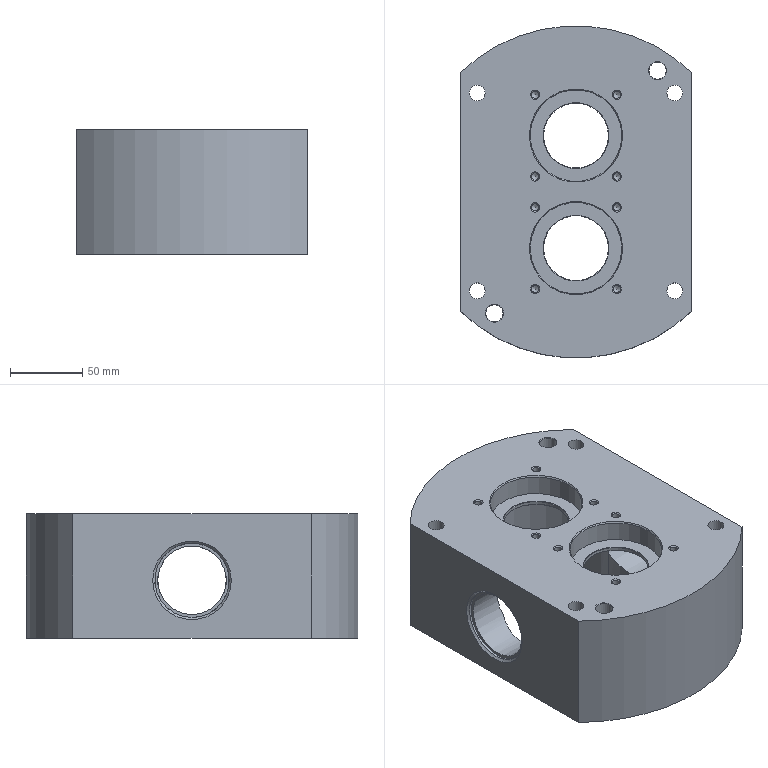NC program | NX | posted with a generic post | part box 160 x 230 x 86 mm
Lines 86 to 894 of 2142:
(HOLE_MILLING_COPY_COPY , TOOL : D10)
N146 T10 M6
N148 G54
N150 G17 G0 G90 X-39. Y0. B0. C0. S3000 M3
N152 G43 Z30. H10
N154 Z0.5
N156 G94 G3 X-40.25 Y-1.25 R1.25 F2200.
N158 X-39. Y-2.5 R1.25
N160 X-39. Y-2.5 Z0.28 I0. J2.5
N162 X-39. Y-2.5 Z0.06 I0. J2.5
N164 X-39. Y-2.5 Z-0.16 I0. J2.5
N166 X-39. Y-2.5 Z-0.38 I0. J2.5
N168 X-39. Y-2.5 Z-0.6 I0. J2.5
N170 X-39. Y-2.5 Z-0.82 I0. J2.5
N172 X-39. Y-2.5 Z-1.04 I0. J2.5
N174 X-39. Y-2.5 Z-1.26 I0. J2.5
N176 X-39. Y-2.5 Z-1.48 I0. J2.5
N178 X-39. Y-2.5 Z-1.7 I0. J2.5
N180 X-39. Y-2.5 Z-1.92 I0. J2.5
N182 X-39. Y-2.5 Z-2.14 I0. J2.5
N184 X-39. Y-2.5 Z-2.36 I0. J2.5
N186 X-39. Y-2.5 Z-2.58 I0. J2.5
N188 X-39. Y-2.5 Z-2.8 I0. J2.5
N190 X-39. Y-2.5 Z-3.02 I0. J2.5
N192 X-39. Y-2.5 Z-3.24 I0. J2.5
N194 X-39. Y-2.5 Z-3.46 I0. J2.5
N196 X-39. Y-2.5 Z-3.68 I0. J2.5
N198 X-39. Y-2.5 Z-3.9 I0. J2.5
N200 X-39. Y-2.5 Z-4.12 I0. J2.5
N202 X-39. Y-2.5 Z-4.34 I0. J2.5
N204 X-39. Y-2.5 Z-4.56 I0. J2.5
N206 X-39. Y-2.5 Z-4.78 I0. J2.5
N208 X-39. Y-2.5 Z-5. I0. J2.5
N210 X-39. Y-2.5 Z-5.22 I0. J2.5
N212 X-39. Y-2.5 Z-5.44 I0. J2.5
N214 X-39. Y-2.5 Z-5.66 I0. J2.5
N216 X-39. Y-2.5 Z-5.88 I0. J2.5
N218 X-39. Y-2.5 Z-6.1 I0. J2.5
N220 X-39. Y-2.5 Z-6.32 I0. J2.5
N222 X-39. Y-2.5 Z-6.54 I0. J2.5
N224 X-39. Y-2.5 Z-6.76 I0. J2.5
N226 X-39. Y-2.5 Z-6.98 I0. J2.5
N228 X-39. Y-2.5 Z-7.2 I0. J2.5
N230 X-39. Y-2.5 Z-7.42 I0. J2.5
N232 X-39. Y-2.5 Z-7.64 I0. J2.5
N234 X-39. Y-2.5 Z-7.86 I0. J2.5
N236 X-39. Y-2.5 Z-8.08 I0. J2.5
N238 X-39. Y-2.5 Z-8.3 I0. J2.5
N240 X-39. Y-2.5 Z-8.52 I0. J2.5
N242 X-39. Y-2.5 Z-8.74 I0. J2.5
N244 X-39. Y-2.5 Z-8.96 I0. J2.5
N246 X-39. Y-2.5 Z-9.18 I0. J2.5
N248 X-39. Y-2.5 Z-9.4 I0. J2.5
N250 X-39. Y-2.5 Z-9.62 I0. J2.5
N252 X-39. Y-2.5 Z-9.84 I0. J2.5
N254 X-39. Y-2.5 Z-10.06 I0. J2.5
N256 X-39. Y-2.5 Z-10.28 I0. J2.5
N258 X-39. Y-2.5 Z-10.5 I0. J2.5
N260 X-39. Y-2.5 Z-10.72 I0. J2.5
N262 X-39. Y-2.5 Z-10.94 I0. J2.5
N264 X-39. Y-2.5 Z-11.16 I0. J2.5
N266 X-39. Y-2.5 Z-11.38 I0. J2.5
N268 X-39. Y-2.5 Z-11.6 I0. J2.5
N270 X-39. Y-2.5 Z-11.82 I0. J2.5
N272 X-39. Y-2.5 Z-12.04 I0. J2.5
N274 X-39. Y-2.5 Z-12.26 I0. J2.5
N276 X-39. Y-2.5 Z-12.48 I0. J2.5
N278 X-39. Y-2.5 Z-12.7 I0. J2.5
N280 X-39. Y-2.5 Z-12.92 I0. J2.5
N282 X-39. Y-2.5 Z-13.14 I0. J2.5
N284 X-39. Y-2.5 Z-13.36 I0. J2.5
N286 X-39. Y-2.5 Z-13.58 I0. J2.5
N288 X-39. Y-2.5 Z-13.8 I0. J2.5
N290 X-39. Y-2.5 Z-14.02 I0. J2.5
N292 X-39. Y-2.5 Z-14.24 I0. J2.5
N294 X-39. Y-2.5 Z-14.46 I0. J2.5
N296 X-39. Y-2.5 Z-14.68 I0. J2.5
N298 X-39. Y-2.5 Z-14.9 I0. J2.5
N300 X-38.296 Y2.399 Z-15. R2.5
N302 X-41.437 Y0.697 R2.535
N304 X-39.765 Y-2.485 R2.565
N306 X-36.477 Y-0.809 R2.617
N308 X-38.173 Y2.569 R2.681
N310 X-41.607 Y0.872 R2.717
N312 X-39.892 Y-2.653 R2.78
N314 X-36.311 Y-0.939 R2.817
N316 X-38.04 Y2.735 R2.88
N318 X-41.771 Y1.007 R2.916
N320 X-40.029 Y-2.816 R2.98
N322 X-36.149 Y-1.078 R3.016
N324 X-37.899 Y2.895 R3.079
N326 X-41.929 Y1.151 R3.115
N328 X-40.175 Y-2.973 R3.179
N330 X-35.993 Y-1.226 R3.215
N332 X-37.748 Y3.05 R3.278
N334 X-42.082 Y1.303 R3.315
N336 X-40.33 Y-3.125 R3.378
N338 X-35.844 Y-1.383 R3.414
N340 X-37.589 Y3.199 R3.478
N342 X-42.229 Y1.464 R3.514
N344 X-40.494 Y-3.271 R3.577
N346 X-35.7 Y-1.548 R3.613
N348 X-37.422 Y3.341 R3.677
N350 X-42.37 Y1.634 R3.713
N352 X-40.665 Y-3.41 R3.776
N354 X-35.563 Y-1.722 R3.813
N356 X-37.246 Y3.477 R3.876
N358 X-42.503 Y1.812 R3.912
N360 X-40.845 Y-3.542 R3.976
N362 X-35.433 Y-1.904 R4.012
N364 X-37.062 Y3.605 R4.075
N366 X-42.63 Y1.997 R4.111
N368 X-41.033 Y-3.667 R4.175
N370 X-35.31 Y-2.093 R4.211
N372 X-36.87 Y3.727 R4.274
N374 X-42.749 Y2.191 R4.311
N376 X-41.229 Y-3.785 R4.374
N378 X-35.194 Y-2.291 R4.41
N380 X-36.671 Y3.84 R4.474
N382 X-42.86 Y2.392 R4.51
N384 X-41.432 Y-3.894 R4.573
N386 X-35.087 Y-2.495 R4.609
N388 X-36.464 Y3.946 R4.673
N390 X-42.964 Y2.6 R4.709
N392 X-41.642 Y-3.996 R4.772
N394 X-34.987 Y-2.707 R4.808
N396 X-36.25 Y4.044 R4.872
N398 X-43.059 Y2.815 R4.908
N400 X-41.859 Y-4.089 R4.971
N402 X-34.897 Y-2.925 R5.008
N404 X-36.03 Y4.133 R5.071
N406 X-43.146 Y3.037 R5.107
N408 X-42.083 Y-4.174 R5.171
N410 X-34.814 Y-3.15 R5.207
N412 X-35.803 Y4.213 R5.27
N414 X-43.223 Y3.265 R5.306
N416 X-42.312 Y-4.25 R5.37
N418 X-34.741 Y-3.381 R5.406
N420 X-35.571 Y4.284 R5.469
N422 X-43.292 Y3.499 R5.506
N424 X-42.548 Y-4.316 R5.569
N426 X-34.678 Y-3.618 R5.605
N428 X-35.332 Y4.346 R5.669
N430 X-43.351 Y3.739 R5.705
N432 X-42.789 Y-4.373 R5.768
N434 X-34.623 Y-3.861 R5.804
N436 X-35.088 Y4.398 R5.868
N438 X-43.4 Y3.984 R5.904
N440 X-43.036 Y-4.42 R5.967
N442 X-34.579 Y-4.108 R6.004
N444 X-34.839 Y4.44 R6.067
N446 X-43.44 Y4.234 R6.103
N448 X-43.287 Y-4.458 R6.167
N450 X-34.544 Y-4.361 R6.203
N452 X-34.585 Y4.472 R6.266
N454 X-43.469 Y4.488 R6.302
N456 X-43.543 Y-4.485 R6.366
N458 X-34.52 Y-4.617 R6.402
N460 X-34.327 Y4.494 R6.465
N462 X-43.488 Y4.747 R6.501
N464 X-43.804 Y-4.501 R6.565
N466 X-34.506 Y-4.878 R6.601
N468 X-34.065 Y4.506 R6.664
N470 X-43.497 Y5.01 R6.701
N472 X-44.068 Y-4.508 R6.764
N474 X-34.503 Y-5.143 R6.8
N476 X-33.799 Y4.507 R6.864
N478 X-43.495 Y5.277 R6.9
N480 X-44.335 Y-4.503 R6.963
N482 X-34.51 Y-5.411 R6.999
N484 X-33.53 Y4.497 R7.063
N486 X-43.482 Y5.546 R7.099
N488 X-44.606 Y-4.487 R7.162
N490 X-34.529 Y-5.682 R7.199
N492 X-33.258 Y4.475 R7.262
N494 X-43.458 Y5.819 R7.298
N496 X-44.879 Y-4.461 R7.362
N498 X-34.559 Y-5.956 R7.398
N500 X-32.984 Y4.443 R7.461
N502 X-43.422 Y6.093 R7.497
N504 X-45.155 Y-4.423 R7.561
N506 X-34.599 Y-6.232 R7.597
N508 X-32.707 Y4.4 R7.66
N510 X-43.376 Y6.37 R7.697
N512 X-45.432 Y-4.374 R7.76
N514 X-34.652 Y-6.509 R7.796
N516 X-32.429 Y4.345 R7.86
N518 X-43.318 Y6.648 R7.896
N520 X-45.711 Y-4.313 R7.959
N522 X-34.716 Y-6.788 R7.995
N524 X-32.149 Y4.278 R8.059
N526 X-43.248 Y6.928 R8.095
N528 X-45.991 Y-4.24 R8.158
N530 X-34.791 Y-7.068 R8.194
N532 X-31.869 Y4.2 R8.258
N534 X-43.167 Y7.208 R8.294
N536 X-46.272 Y-4.156 R8.357
N538 X-34.878 Y-7.348 R8.394
N540 X-31.588 Y4.11 R8.457
N542 X-43.074 Y7.489 R8.493
N544 X-46.552 Y-4.061 R8.557
N546 X-34.977 Y-7.629 R8.593
N548 X-31.307 Y4.008 R8.656
N550 X-42.969 Y7.769 R8.692
N552 X-46.833 Y-3.953 R8.756
N554 X-35.088 Y-7.909 R8.792
N556 X-31.027 Y3.895 R8.855
N558 X-42.852 Y8.049 R8.892
N560 X-47.113 Y-3.833 R8.955
N562 X-35.211 Y-8.189 R8.991
N564 X-30.747 Y3.769 R9.055
N566 X-42.723 Y8.328 R9.091
N568 X-47.392 Y-3.702 R9.154
N570 X-35.346 Y-8.467 R9.19
N572 X-30.469 Y3.631 R9.254
N574 X-42.583 Y8.606 R9.29
N576 X-47.67 Y-3.558 R9.353
N578 X-35.492 Y-8.744 R9.39
N580 X-30.192 Y3.482 R9.453
N582 X-42.43 Y8.881 R9.489
N584 X-47.945 Y-3.403 R9.553
N586 X-35.651 Y-9.019 R9.589
N588 X-29.918 Y3.321 R9.652
N590 X-42.266 Y9.155 R9.688
N592 X-48.219 Y-3.235 R9.752
N594 X-35.821 Y-9.291 R9.788
N596 X-29.646 Y3.147 R9.851
N598 X-42.089 Y9.426 R9.887
N600 X-48.489 Y-3.056 R9.951
N602 X-36.004 Y-9.56 R9.987
N604 X-29.377 Y2.962 R10.05
N606 X-41.901 Y9.694 R10.087
N608 X-48.756 Y-2.865 R10.15
N610 X-36.198 Y-9.826 R10.186
N612 X-29.111 Y2.765 R10.25
N614 X-41.7 Y9.958 R10.286
N616 X-49.02 Y-2.662 R10.349
N618 X-36.404 Y-10.089 R10.385
N620 X-28.85 Y2.556 R10.449
N622 X-41.488 Y10.218 R10.485
N624 X-49.279 Y-2.447 R10.548
N626 X-36.622 Y-10.347 R10.585
N628 X-28.593 Y2.335 R10.648
N630 X-41.265 Y10.474 R10.684
N632 X-49.534 Y-2.22 R10.748
N634 X-36.852 Y-10.6 R10.784
N636 X-28.34 Y2.102 R10.847
N638 X-41.029 Y10.725 R10.883
N640 X-49.784 Y-1.982 R10.947
N642 X-37.093 Y-10.848 R10.983
N644 X-28.093 Y1.858 R11.046
N646 X-40.782 Y10.97 R11.082
N648 X-50.029 Y-1.732 R11.146
N650 X-37.345 Y-11.091 R11.182
N652 X-27.851 Y1.603 R11.246
N654 X-40.524 Y11.21 R11.282
N656 X-50.268 Y-1.471 R11.345
N658 X-37.609 Y-11.328 R11.381
N660 X-27.615 Y1.336 R11.445
N662 X-40.254 Y11.444 R11.481
N664 X-50.5 Y-1.199 R11.544
N666 X-37.885 Y-11.558 R11.58
N668 X-27.386 Y1.058 R11.644
N670 X-39.974 Y11.671 R11.68
N672 X-50.726 Y-0.915 R11.743
N674 X-38.171 Y-11.782 R11.78
N676 X-27.164 Y0.769 R11.843
N678 X-39.682 Y11.891 R11.879
N680 X-50.945 Y-0.621 R11.943
N682 X-38.468 Y-11.999 R11.979
N684 X-26.949 Y0.47 R12.042
N686 X-39.379 Y12.104 R12.078
N688 X-51.156 Y-0.316 R12.142
N690 X-38.776 Y-12.208 R12.178
N692 X-26.742 Y0.159 R12.241
N694 X-39.066 Y12.309 R12.278
N696 X-51.359 Y0. R12.341
N698 X-39.094 Y-12.409 R12.377
N700 X-26.542 Y-0.162 R12.441
N702 X-38.743 Y12.506 R12.477
N704 X-51.554 Y0.326 R12.54
N706 X-39.423 Y-12.601 R12.576
N708 X-26.352 Y-0.493 R12.64
N710 X-38.409 Y12.694 R12.676
N712 X-51.74 Y0.662 R12.739
N714 X-39.761 Y-12.785 R12.775
N716 X-26.17 Y-0.834 R12.839
N718 X-38.066 Y12.873 R12.875
N720 X-51.917 Y1.008 R12.938
N722 X-40.11 Y-12.959 R12.975
N724 X-25.998 Y-1.185 R13.038
N726 X-37.712 Y13.043 R13.074
N728 X-52.085 Y1.364 R13.138
N730 X-40.468 Y-13.124 R13.174
N732 X-25.835 Y-1.545 R13.237
N734 X-37.35 Y13.202 R13.273
N736 X-52.243 Y1.729 R13.337
N738 X-40.835 Y-13.279 R13.373
N740 X-25.682 Y-1.915 R13.436
N742 X-36.978 Y13.352 R13.473
N744 X-52.39 Y2.103 R13.536
N746 X-41.211 Y-13.423 R13.572
N748 X-25.54 Y-2.293 R13.636
N750 X-36.597 Y13.491 R13.672
N752 X-52.527 Y2.486 R13.735
N754 X-41.596 Y-13.557 R13.771
N756 X-25.409 Y-2.681 R13.835
N758 X-36.208 Y13.619 R13.871
N760 X-52.653 Y2.877 R13.934
N762 X-41.99 Y-13.679 R13.971
N764 X-25.289 Y-3.076 R14.034
N766 X-35.811 Y13.736 R14.07
N768 X-52.767 Y3.277 R14.134
N770 X-42.391 Y-13.791 R14.17
N772 X-25.18 Y-3.48 R14.233
N774 X-35.405 Y13.842 R14.269
N776 X-52.87 Y3.684 R14.333
N778 X-42.8 Y-13.89 R14.369
N780 X-25.083 Y-3.891 R14.432
N782 X-34.992 Y13.935 R14.468
N784 X-52.961 Y4.099 R14.532
N786 X-43.217 Y-13.977 R14.568
N788 X-24.999 Y-4.309 R14.631
N790 X-34.572 Y14.017 R14.668
N792 X-53.039 Y4.521 R14.731
N794 X-43.641 Y-14.052 R14.767
N796 X-24.926 Y-4.735 R14.831
N798 X-34.145 Y14.085 R14.867
N800 X-53.105 Y4.95 R14.93
N802 X-44.071 Y-14.115 R14.966
N804 X-24.867 Y-5.167 R15.03
N806 X-33.711 Y14.141 R15.066
N808 X-53.158 Y5.386 R15.129
N810 X-44.508 Y-14.164 R15.166
N812 X-24.821 Y-5.605 R15.229
N814 X-33.271 Y14.184 R15.265
N816 X-53.197 Y5.827 R15.329
N818 X-44.951 Y-14.2 R15.365
N820 X-24.788 Y-6.05 R15.428
N822 X-32.826 Y14.213 R15.464
N824 X-53.224 Y6.274 R15.528
N826 X-45.399 Y-14.222 R15.564
N828 X-24.768 Y-6.499 R15.627
N830 X-32.375 Y14.229 R15.664
N832 X-53.236 Y6.726 R15.727
N834 X-45.852 Y-14.231 R15.763
N836 X-24.763 Y-6.954 R15.827
N838 X-31.919 Y14.23 R15.863
N840 X-53.234 Y7.183 R15.926
N842 X-46.31 Y-14.226 R15.962
N844 X-24.772 Y-7.413 R16.026
N846 X-31.459 Y14.218 R16.062
N848 X-53.219 Y7.645 R16.125
N850 X-46.772 Y-14.206 R16.161
N852 X-24.795 Y-7.877 R16.225
N854 X-30.995 Y14.191 R16.261
N856 X-53.188 Y8.11 R16.324
N858 X-47.239 Y-14.172 R16.361
N860 X-24.832 Y-8.344 R16.424
N862 X-30.527 Y14.149 R16.46
N864 X-53.143 Y8.579 R16.524
N866 X-47.708 Y-14.123 R16.56
N868 X-24.885 Y-8.814 R16.623
N870 X-30.056 Y14.092 R16.659
N872 X-53.083 Y9.051 R16.723
N874 X-48.181 Y-14.059 R16.759
N876 X-24.952 Y-9.288 R16.822
N878 X-29.582 Y14.021 R16.859
N880 X-53.008 Y9.525 R16.922
N882 X-48.656 Y-13.98 R16.958
N884 X-25.035 Y-9.763 R17.022
N886 X-29.106 Y13.934 R17.058
N888 X-52.918 Y10.002 R17.121
N890 X-49.132 Y-13.885 R17.157
N892 X-25.133 Y-10.241 R17.221
N894 X-28.628 Y13.832 R17.257
N896 X-52.812 Y10.48 R17.32
N898 X-49.611 Y-13.775 R17.356
N900 X-25.246 Y-10.72 R17.42
N902 X-28.149 Y13.715 R17.456
N904 X-52.691 Y10.96 R17.519
N906 X-50.09 Y-13.65 R17.556
N908 X-25.375 Y-11.2 R17.619
N910 X-27.67 Y13.581 R17.655
N912 X-52.554 Y11.44 R17.719
N914 X-50.571 Y-13.509 R17.755
N916 X-25.52 Y-11.68 R17.818
N918 X-27.189 Y13.432 R17.854
N920 X-52.401 Y11.921 R17.918
N922 X-51.051 Y-13.352 R17.954
N924 X-25.681 Y-12.161 R18.017
N926 X-26.709 Y13.267 R18.054
N928 X-52.233 Y12.401 R18.117
N930 X-51.53 Y-13.179 R18.153
N932 X-25.857 Y-12.64 R18.217
N934 X-26.23 Y13.086 R18.253
N936 X-52.048 Y12.88 R18.316
N938 X-52.009 Y-12.99 R18.352
N940 X-26.05 Y-13.119 R18.416
N942 X-25.752 Y12.889 R18.452
N944 X-51.847 Y13.358 R18.515
N946 X-52.486 Y-12.785 R18.552
N948 X-26.259 Y-13.596 R18.615
N950 X-25.276 Y12.676 R18.651
N952 X-51.631 Y13.834 R18.715
N954 X-52.962 Y-12.564 R18.751
N956 X-26.484 Y-14.071 R18.814
N958 X-24.802 Y12.447 R18.85
N960 X-51.398 Y14.308 R18.914
N962 X-53.435 Y-12.327 R18.95
N964 X-26.725 Y-14.544 R19.013
N966 X-24.33 Y12.202 R19.049
N968 X-51.149 Y14.779 R19.113
N970 X-53.904 Y-12.073 R19.149
N972 X-26.982 Y-15.013 R19.212
N974 X-23.862 Y11.94 R19.249
N976 X-50.883 Y15.246 R19.312
N978 X-54.371 Y-11.804 R19.348
N980 X-27.255 Y-15.478 R19.412
N982 X-23.398 Y11.663 R19.448
N984 X-50.602 Y15.71 R19.511
N986 X-54.833 Y-11.518 R19.547
N988 X-27.545 Y-15.94 R19.611
N990 X-22.938 Y11.369 R19.647
N992 X-50.304 Y16.169 R19.71
N994 X-55.291 Y-11.216 R19.747
N996 X-27.851 Y-16.397 R19.81
N998 X-22.483 Y11.059 R19.846
N1000 X-49.99 Y16.623 R19.91
N1002 X-55.743 Y-10.898 R19.946
N1004 X-28.172 Y-16.848 R20.009
N1006 X-22.033 Y10.733 R20.045
N1008 X-49.661 Y17.072 R20.109
N1010 X-56.19 Y-10.564 R20.145
N1012 X-28.51 Y-17.294 R20.208
N1014 X-21.589 Y10.391 R20.245
N1016 X-49.315 Y17.514 R20.308
N1018 X-56.631 Y-10.214 R20.344
N1020 X-28.864 Y-17.733 R20.408
N1022 X-21.151 Y10.033 R20.444
N1024 X-48.953 Y17.95 R20.507
N1026 X-57.065 Y-9.849 R20.543
N1028 X-29.233 Y-18.166 R20.607
N1030 X-20.721 Y9.66 R20.643
N1032 X-48.576 Y18.379 R20.706
N1034 X-57.492 Y-9.467 R20.742
N1036 X-29.618 Y-18.591 R20.806
N1038 X-20.298 Y9.271 R20.842
N1040 X-48.183 Y18.801 R20.905
N1042 X-57.911 Y-9.07 R20.942
N1044 X-30.019 Y-19.008 R21.005
N1046 X-19.883 Y8.866 R21.041
N1048 X-47.775 Y19.214 R21.105
N1050 X-58.321 Y-8.658 R21.141
N1052 X-30.435 Y-19.417 R21.204
N1054 X-19.476 Y8.446 R21.24
N1056 X-47.351 Y19.618 R21.304
N1058 X-58.723 Y-8.23 R21.34
N1060 X-30.867 Y-19.817 R21.403
N1062 X-19.079 Y8.011 R21.44
N1064 X-46.912 Y20.014 R21.503
N1066 X-59.116 Y-7.787 R21.539
N1068 X-31.313 Y-20.208 R21.603
N1070 X-18.691 Y7.56 R21.639
N1072 X-46.458 Y20.4 R21.702
N1074 X-59.499 Y-7.33 R21.738
N1076 X-31.774 Y-20.589 R21.802
N1078 X-18.313 Y7.095 R21.838
N1080 X-45.99 Y20.775 R21.901
N1082 X-59.872 Y-6.857 R21.937
N1084 X-32.25 Y-20.959 R22.001
N1086 X-17.946 Y6.616 R22.037
N1088 X-45.507 Y21.14 R22.1
N1090 X-60.233 Y-6.371 R22.137
N1092 X-32.74 Y-21.318 R22.2
N1094 X-17.59 Y6.122 R22.236
N1096 X-45.009 Y21.494 R22.3
N1098 X-60.584 Y-5.87 R22.336
N1100 X-33.245 Y-21.666 R22.399
N1102 X-17.246 Y5.614 R22.435
N1104 X-44.498 Y21.835 R22.499
N1106 X-60.922 Y-5.355 R22.535
N1108 X-33.763 Y-22.002 R22.598
N1110 X-16.913 Y5.092 R22.635
N1112 X-43.973 Y22.165 R22.698
N1114 X-61.248 Y-4.826 R22.734
N1116 X-34.295 Y-22.325 R22.798
N1118 X-16.593 Y4.557 R22.834
N1120 X-43.434 Y22.482 R22.897
N1122 X-61.562 Y-4.284 R22.933
N1124 X-34.84 Y-22.636 R22.997
N1126 X-16.286 Y4.008 R23.033
N1128 X-42.882 Y22.786 R23.096
N1130 X-61.862 Y-3.729 R23.133
N1132 X-35.398 Y-22.933 R23.196
N1134 X-15.993 Y3.447 R23.232
N1136 X-42.318 Y23.076 R23.296
N1138 X-62.149 Y-3.161 R23.332
N1140 X-35.969 Y-23.216 R23.395
N1142 X-15.714 Y2.873 R23.431
N1144 X-41.741 Y23.353 R23.495
N1146 X-62.421 Y-2.581 R23.531
N1148 X-36.552 Y-23.485 R23.594
N1150 X-15.449 Y2.287 R23.63
N1152 X-41.152 Y23.614 R23.694
N1154 X-62.678 Y-1.989 R23.73
N1156 X-37.147 Y-23.739 R23.793
N1158 X-15.198 Y1.689 R23.83
N1160 X-40.551 Y23.861 R23.893
N1162 X-62.921 Y-1.385 R23.929
N1164 X-37.754 Y-23.978 R23.993
N1166 X-14.964 Y1.079 R24.029
N1168 X-39.939 Y24.092 R24.092
N1170 X-63.148 Y-0.77 R24.128
N1172 X-38.371 Y-24.202 R24.192
N1174 X-14.745 Y0.459 R24.228
N1176 X-39.316 Y24.307 R24.291
N1178 X-63.359 Y-0.145 R24.328
N1180 X-39. Y-24.409 R24.391
N1182 X-14.542 Y-0.172 R24.427
N1184 X-38.682 Y24.507 R24.491
N1186 X-63.554 Y0.492 R24.527
N1188 X-39.639 Y-24.6 R24.59
N1190 X-14.355 Y-0.814 R24.626
N1192 X-38.038 Y24.689 R24.69
N1194 X-63.731 Y1.138 R24.726
N1196 X-40.288 Y-24.774 R24.789
N1198 X-14.186 Y-1.465 R24.825
N1200 X-37.384 Y24.855 R24.889
N1202 X-63.892 Y1.794 R24.925
N1204 X-40.946 Y-24.931 R24.989
N1206 X-14.034 Y-2.125 R25.025
N1208 X-36.722 Y25.003 R25.088
N1210 X-64.036 Y2.459 R25.124
N1212 X-41.613 Y-25.07 R25.188
N1214 X-13.9 Y-2.795 R25.224
N1216 X-36.05 Y25.133 R25.287
N1218 X-64.161 Y3.132 R25.323
N1220 X-42.289 Y-25.191 R25.387
N1222 X-13.783 Y-3.472 R25.423
N1224 X-35.37 Y25.245 R25.486
N1226 X-64.268 Y3.814 R25.523
N1228 X-42.973 Y-25.294 R25.586
N1230 X-13.685 Y-4.158 R25.622
N1232 X-34.683 Y25.339 R25.686
N1234 X-64.357 Y4.504 R25.722
N1236 X-43.664 Y-25.378 R25.785
N1238 X-13.606 Y-4.851 R25.821
N1240 X-33.988 Y25.413 R25.885
N1242 X-64.426 Y5.2 R25.921
N1244 X-44.362 Y-25.444 R25.984
N1246 X-13.546 Y-5.551 R26.021
N1248 X-33.286 Y25.469 R26.084
N1250 X-64.477 Y5.903 R26.12
N1252 X-45.067 Y-25.49 R26.184
N1254 X-13.505 Y-6.257 R26.22
N1256 X-32.578 Y25.505 R26.283
N1258 X-64.508 Y6.613 R26.319
N1260 X-45.778 Y-25.516 R26.383
N1262 X-13.484 Y-6.969 R26.419
N1264 X-31.865 Y25.522 R26.482
N1266 X-64.547 Y7.286 R26.534
N1268 X-46.494 Y-25.523 R26.566
N1270 X-13.477 Y-7.494 R26.6
N1272 X-46.494 Y-25.523 R-26.6
N1274 X-29.986 Y-16.508 R13.3
N1276 X-39. Y0. R13.3
N1278 G0 Z30.
N1280 X39.
N1282 Z0.5
N1284 G3 X37.75 Y-1.25 R1.25
N1286 X39. Y-2.5 R1.25
N1288 X39. Y-2.5 Z0.28 I0. J2.5
N1290 X39. Y-2.5 Z0.06 I0. J2.5
N1292 X39. Y-2.5 Z-0.16 I0. J2.5
N1294 X39. Y-2.5 Z-0.38 I0. J2.5
N1296 X39. Y-2.5 Z-0.6 I0. J2.5
N1298 X39. Y-2.5 Z-0.82 I0. J2.5
N1300 X39. Y-2.5 Z-1.04 I0. J2.5
N1302 X39. Y-2.5 Z-1.26 I0. J2.5
N1304 X39. Y-2.5 Z-1.48 I0. J2.5
N1306 X39. Y-2.5 Z-1.7 I0. J2.5
N1308 X39. Y-2.5 Z-1.92 I0. J2.5
N1310 X39. Y-2.5 Z-2.14 I0. J2.5
N1312 X39. Y-2.5 Z-2.36 I0. J2.5
N1314 X39. Y-2.5 Z-2.58 I0. J2.5
N1316 X39. Y-2.5 Z-2.8 I0. J2.5
N1318 X39. Y-2.5 Z-3.02 I0. J2.5
N1320 X39. Y-2.5 Z-3.24 I0. J2.5
N1322 X39. Y-2.5 Z-3.46 I0. J2.5
N1324 X39. Y-2.5 Z-3.68 I0. J2.5
N1326 X39. Y-2.5 Z-3.9 I0. J2.5
N1328 X39. Y-2.5 Z-4.12 I0. J2.5
N1330 X39. Y-2.5 Z-4.34 I0. J2.5
N1332 X39. Y-2.5 Z-4.56 I0. J2.5
N1334 X39. Y-2.5 Z-4.78 I0. J2.5
N1336 X39. Y-2.5 Z-5. I0. J2.5
N1338 X39. Y-2.5 Z-5.22 I0. J2.5
N1340 X39. Y-2.5 Z-5.44 I0. J2.5
N1342 X39. Y-2.5 Z-5.66 I0. J2.5
N1344 X39. Y-2.5 Z-5.88 I0. J2.5
N1346 X39. Y-2.5 Z-6.1 I0. J2.5
N1348 X39. Y-2.5 Z-6.32 I0. J2.5
N1350 X39. Y-2.5 Z-6.54 I0. J2.5
N1352 X39. Y-2.5 Z-6.76 I0. J2.5
N1354 X39. Y-2.5 Z-6.98 I0. J2.5
N1356 X39. Y-2.5 Z-7.2 I0. J2.5
N1358 X39. Y-2.5 Z-7.42 I0. J2.5
N1360 X39. Y-2.5 Z-7.64 I0. J2.5
N1362 X39. Y-2.5 Z-7.86 I0. J2.5
N1364 X39. Y-2.5 Z-8.08 I0. J2.5
N1366 X39. Y-2.5 Z-8.3 I0. J2.5
N1368 X39. Y-2.5 Z-8.52 I0. J2.5
N1370 X39. Y-2.5 Z-8.74 I0. J2.5
N1372 X39. Y-2.5 Z-8.96 I0. J2.5
N1374 X39. Y-2.5 Z-9.18 I0. J2.5
N1376 X39. Y-2.5 Z-9.4 I0. J2.5
N1378 X39. Y-2.5 Z-9.62 I0. J2.5
N1380 X39. Y-2.5 Z-9.84 I0. J2.5
N1382 X39. Y-2.5 Z-10.06 I0. J2.5
N1384 X39. Y-2.5 Z-10.28 I0. J2.5
N1386 X39. Y-2.5 Z-10.5 I0. J2.5
N1388 X39. Y-2.5 Z-10.72 I0. J2.5
N1390 X39. Y-2.5 Z-10.94 I0. J2.5
N1392 X39. Y-2.5 Z-11.16 I0. J2.5
N1394 X39. Y-2.5 Z-11.38 I0. J2.5
N1396 X39. Y-2.5 Z-11.6 I0. J2.5
N1398 X39. Y-2.5 Z-11.82 I0. J2.5
N1400 X39. Y-2.5 Z-12.04 I0. J2.5
N1402 X39. Y-2.5 Z-12.26 I0. J2.5
N1404 X39. Y-2.5 Z-12.48 I0. J2.5
N1406 X39. Y-2.5 Z-12.7 I0. J2.5
N1408 X39. Y-2.5 Z-12.92 I0. J2.5
N1410 X39. Y-2.5 Z-13.14 I0. J2.5
N1412 X39. Y-2.5 Z-13.36 I0. J2.5
N1414 X39. Y-2.5 Z-13.58 I0. J2.5
N1416 X39. Y-2.5 Z-13.8 I0. J2.5
N1418 X39. Y-2.5 Z-14.02 I0. J2.5
N1420 X39. Y-2.5 Z-14.24 I0. J2.5
N1422 X39. Y-2.5 Z-14.46 I0. J2.5
N1424 X39. Y-2.5 Z-14.68 I0. J2.5
N1426 X39. Y-2.5 Z-14.9 I0. J2.5
N1428 X39.704 Y2.399 Z-15. R2.5
N1430 X36.563 Y0.697 R2.535
N1432 X38.235 Y-2.485 R2.565
N1434 X41.523 Y-0.809 R2.617
N1436 X39.827 Y2.569 R2.681
N1438 X36.393 Y0.872 R2.717
N1440 X38.108 Y-2.653 R2.78
N1442 X41.689 Y-0.939 R2.817
N1444 X39.96 Y2.735 R2.88
N1446 X36.229 Y1.007 R2.916
N1448 X37.971 Y-2.816 R2.98
N1450 X41.851 Y-1.078 R3.016
N1452 X40.101 Y2.895 R3.079
N1454 X36.071 Y1.151 R3.115
N1456 X37.825 Y-2.973 R3.179
N1458 X42.007 Y-1.226 R3.215
N1460 X40.252 Y3.05 R3.278
N1462 X35.918 Y1.303 R3.315
N1464 X37.67 Y-3.125 R3.378
N1466 X42.156 Y-1.383 R3.414
N1468 X40.411 Y3.199 R3.478
N1470 X35.771 Y1.464 R3.514
N1472 X37.506 Y-3.271 R3.577
N1474 X42.3 Y-1.548 R3.613
N1476 X40.578 Y3.341 R3.677
N1478 X35.63 Y1.634 R3.713
N1480 X37.335 Y-3.41 R3.776
N1482 X42.437 Y-1.722 R3.813
N1484 X40.754 Y3.477 R3.876
N1486 X35.497 Y1.812 R3.912
N1488 X37.155 Y-3.542 R3.976
N1490 X42.567 Y-1.904 R4.012
N1492 X40.938 Y3.605 R4.075
N1494 X35.37 Y1.997 R4.111
N1496 X36.967 Y-3.667 R4.175
N1498 X42.69 Y-2.093 R4.211
N1500 X41.13 Y3.727 R4.274
N1502 X35.251 Y2.191 R4.311
N1504 X36.771 Y-3.785 R4.374
N1506 X42.806 Y-2.291 R4.41
N1508 X41.33 Y3.84 R4.474
N1510 X35.14 Y2.392 R4.51
N1512 X36.568 Y-3.894 R4.573
N1514 X42.913 Y-2.495 R4.609
N1516 X41.536 Y3.946 R4.673
N1518 X35.036 Y2.6 R4.709
N1520 X36.358 Y-3.996 R4.772
N1522 X43.013 Y-2.707 R4.808
N1524 X41.75 Y4.044 R4.872
N1526 X34.941 Y2.815 R4.908
N1528 X36.141 Y-4.089 R4.971
N1530 X43.103 Y-2.925 R5.008
N1532 X41.97 Y4.133 R5.071
N1534 X34.854 Y3.037 R5.107
N1536 X35.917 Y-4.174 R5.171
N1538 X43.186 Y-3.15 R5.207
N1540 X42.197 Y4.213 R5.27
N1542 X34.777 Y3.265 R5.306
N1544 X35.688 Y-4.25 R5.37
N1546 X43.259 Y-3.381 R5.406
N1548 X42.429 Y4.284 R5.469
N1550 X34.708 Y3.499 R5.506
N1552 X35.452 Y-4.316 R5.569
N1554 X43.322 Y-3.618 R5.605
N1556 X42.668 Y4.346 R5.669
N1558 X34.649 Y3.739 R5.705
N1560 X35.211 Y-4.373 R5.768
N1562 X43.377 Y-3.861 R5.804
N1564 X42.912 Y4.398 R5.868
N1566 X34.6 Y3.984 R5.904
N1568 X34.964 Y-4.42 R5.967
N1570 X43.421 Y-4.108 R6.004
N1572 X43.161 Y4.44 R6.067
N1574 X34.56 Y4.234 R6.103
N1576 X34.713 Y-4.458 R6.167
N1578 X43.456 Y-4.361 R6.203
N1580 X43.415 Y4.472 R6.266
N1582 X34.531 Y4.488 R6.302
N1584 X34.457 Y-4.485 R6.366
N1586 X43.48 Y-4.617 R6.402
N1588 X43.673 Y4.494 R6.465
N1590 X34.512 Y4.747 R6.501
N1592 X34.196 Y-4.501 R6.565
N1594 X43.494 Y-4.878 R6.601
N1596 X43.935 Y4.506 R6.664
N1598 X34.503 Y5.01 R6.701
N1600 X33.932 Y-4.508 R6.764
N1602 X43.497 Y-5.143 R6.8
N1604 X44.201 Y4.507 R6.864
N1606 X34.505 Y5.277 R6.9
N1608 X33.665 Y-4.503 R6.963
N1610 X43.49 Y-5.411 R6.999
N1612 X44.47 Y4.497 R7.063
N1614 X34.518 Y5.546 R7.099
N1616 X33.394 Y-4.487 R7.162
N1618 X43.471 Y-5.682 R7.199
N1620 X44.742 Y4.475 R7.262
N1622 X34.542 Y5.819 R7.298
N1624 X33.121 Y-4.461 R7.362
N1626 X43.441 Y-5.956 R7.398
N1628 X45.016 Y4.443 R7.461
N1630 X34.578 Y6.093 R7.497
N1632 X32.845 Y-4.423 R7.561
N1634 X43.401 Y-6.232 R7.597
N1636 X45.293 Y4.4 R7.66
N1638 X34.624 Y6.37 R7.697
N1640 X32.568 Y-4.374 R7.76
N1642 X43.348 Y-6.509 R7.796
N1644 X45.571 Y4.345 R7.86
N1646 X34.682 Y6.648 R7.896
N1648 X32.289 Y-4.313 R7.959
N1650 X43.284 Y-6.788 R7.995
N1652 X45.851 Y4.278 R8.059
N1654 X34.752 Y6.928 R8.095
N1656 X32.009 Y-4.24 R8.158
N1658 X43.209 Y-7.068 R8.194
N1660 X46.131 Y4.2 R8.258
N1662 X34.833 Y7.208 R8.294
N1664 X31.728 Y-4.156 R8.357
N1666 X43.122 Y-7.348 R8.394
N1668 X46.412 Y4.11 R8.457
N1670 X34.926 Y7.489 R8.493
N1672 X31.448 Y-4.061 R8.557
N1674 X43.023 Y-7.629 R8.593
N1676 X46.693 Y4.008 R8.656
N1678 X35.031 Y7.769 R8.692
N1680 X31.167 Y-3.953 R8.756
N1682 X42.912 Y-7.909 R8.792
N1684 X46.973 Y3.895 R8.855
N1686 X35.148 Y8.049 R8.892
N1688 X30.887 Y-3.833 R8.955
N1690 X42.789 Y-8.189 R8.991
N1692 X47.253 Y3.769 R9.055
N1694 X35.277 Y8.328 R9.091
N1696 X30.608 Y-3.702 R9.154
N1698 X42.654 Y-8.467 R9.19
N1700 X47.531 Y3.631 R9.254
N1702 X35.417 Y8.606 R9.29
N1704 X30.33 Y-3.558 R9.353
N1706 X42.508 Y-8.744 R9.39
N1708 X47.808 Y3.482 R9.453
N1710 X35.57 Y8.881 R9.489
N1712 X30.055 Y-3.403 R9.553
N1714 X42.349 Y-9.019 R9.589
N1716 X48.082 Y3.321 R9.652
N1718 X35.734 Y9.155 R9.688
N1720 X29.781 Y-3.235 R9.752
N1722 X42.179 Y-9.291 R9.788
N1724 X48.354 Y3.147 R9.851
N1726 X35.911 Y9.426 R9.887
N1728 X29.511 Y-3.056 R9.951
N1730 X41.996 Y-9.56 R9.987
N1732 X48.623 Y2.962 R10.05
N1734 X36.099 Y9.694 R10.087
N1736 X29.244 Y-2.865 R10.15
N1738 X41.802 Y-9.826 R10.186
N1740 X48.889 Y2.765 R10.25
N1742 X36.3 Y9.958 R10.286
N1744 X28.98 Y-2.662 R10.349
N1746 X41.596 Y-10.089 R10.385
N1748 X49.15 Y2.556 R10.449
N1750 X36.512 Y10.218 R10.485
N1752 X28.721 Y-2.447 R10.548
N1754 X41.378 Y-10.347 R10.585
N1756 X49.407 Y2.335 R10.648